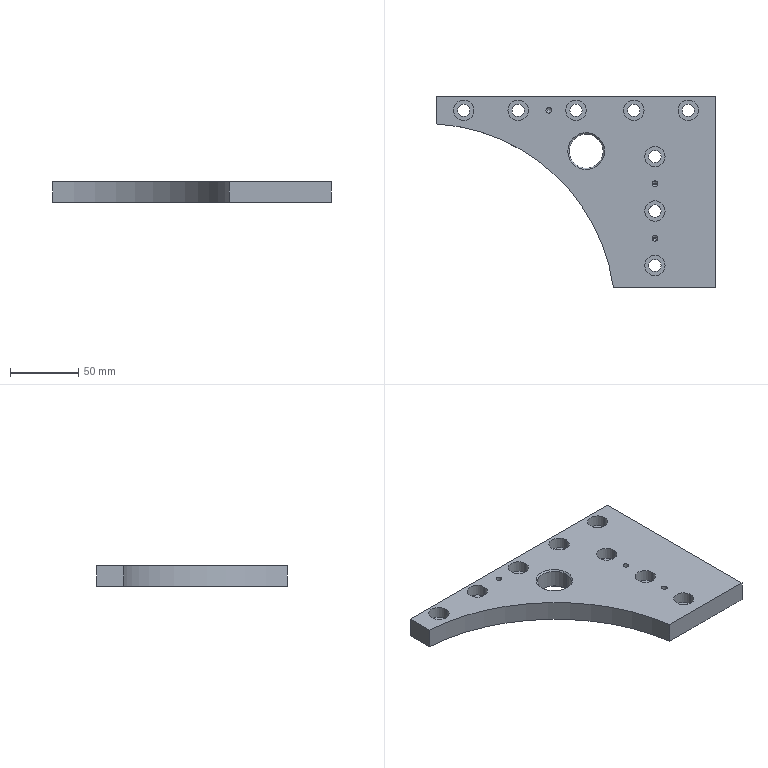Part | SolidWorks | features Cut 2, HoleWzd 2, Chamfer 1, Extrusion 1, Fillet 1, ICE 1 | 1 solid | 65 faces | box 205 x 140 x 15 mm | volume 233014 mm3 | cylinder 41 | plane 14 | cone 10 | commonest cylinder face diameters 9 x16 15 x16 4.2 x6 25 x2 280 x1